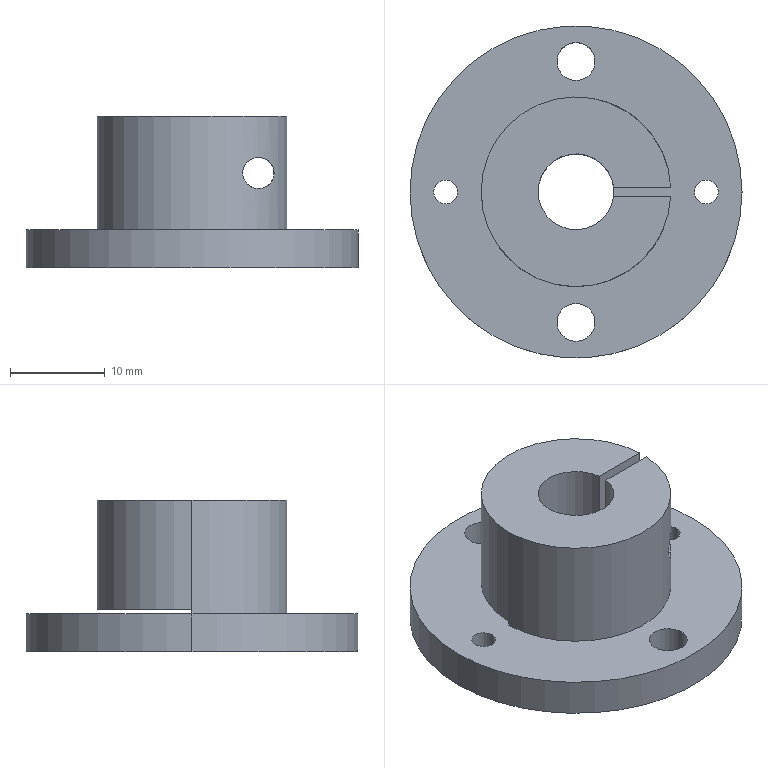Part | STEP file | 11-FG-B04611 | 1 solid | 30 faces | box 35 x 35 x 16 mm | volume 6298 mm3 | cylinder 22 | plane 8 | commonest cylinder face diameters 8 x6 2.5 x4 4 x4 3.3 x2 4.5 x2 20 x2
STEP:
#1=CARTESIAN_POINT('',(12.5,0.,4.));
#2=VERTEX_POINT('',#1);
#3=CARTESIAN_POINT('',(15.,0.,4.));
#4=VERTEX_POINT('',#3);
#5=CARTESIAN_POINT('',(13.75,0.,4.));
#6=DIRECTION('',(0.,0.,1.));
#7=DIRECTION('',(1.,0.,0.));
#8=AXIS2_PLACEMENT_3D('',#5,#6,#7);
#9=CIRCLE('',#8,1.25);
#10=EDGE_CURVE('',#2,#4,#9,.T.);
#11=ORIENTED_EDGE('',*,*,#10,.T.);
#12=CARTESIAN_POINT('',(15.,0.,0.));
#13=VERTEX_POINT('',#12);
#14=CARTESIAN_POINT('',(15.,0.,0.));
#15=DIRECTION('',(0.,0.,-1.));
#16=VECTOR('',#15,1000.);
#17=LINE('',#14,#16);
#18=EDGE_CURVE('',#4,#13,#17,.T.);
#19=ORIENTED_EDGE('',*,*,#18,.T.);
#20=CARTESIAN_POINT('',(12.5,0.,0.));
#21=VERTEX_POINT('',#20);
#22=CARTESIAN_POINT('',(13.75,0.,0.));
#23=DIRECTION('',(0.,0.,-1.));
#24=DIRECTION('',(-1.,0.,0.));
#25=AXIS2_PLACEMENT_3D('',#22,#23,#24);
#26=CIRCLE('',#25,1.25);
#27=EDGE_CURVE('',#13,#21,#26,.T.);
#28=ORIENTED_EDGE('',*,*,#27,.T.);
#29=CARTESIAN_POINT('',(12.5,0.,0.));
#30=DIRECTION('',(0.,0.,-1.));
#31=VECTOR('',#30,1000.);
#32=LINE('',#29,#31);
#33=EDGE_CURVE('',#2,#21,#32,.T.);
#34=ORIENTED_EDGE('',*,*,#33,.F.);
#35=EDGE_LOOP('',(#11,#19,#28,#34));
#36=FACE_OUTER_BOUND('',#35,.T.);
#37=CARTESIAN_POINT('',(13.75,0.,0.));
#38=DIRECTION('',(0.,0.,-1.));
#39=DIRECTION('',(-1.,0.,0.));
#40=AXIS2_PLACEMENT_3D('',#37,#38,#39);
#41=CYLINDRICAL_SURFACE('',#40,1.25);
#42=ADVANCED_FACE('',(#36),#41,.F.);
#43=CARTESIAN_POINT('',(-15.,0.,4.));
#44=VERTEX_POINT('',#43);
#45=CARTESIAN_POINT('',(-12.5,0.,4.));
#46=VERTEX_POINT('',#45);
#47=CARTESIAN_POINT('',(-13.75,0.,4.));
#48=DIRECTION('',(0.,0.,1.));
#49=DIRECTION('',(1.,0.,0.));
#50=AXIS2_PLACEMENT_3D('',#47,#48,#49);
#51=CIRCLE('',#50,1.25);
#52=EDGE_CURVE('',#44,#46,#51,.T.);
#53=ORIENTED_EDGE('',*,*,#52,.T.);
#54=CARTESIAN_POINT('',(-12.5,0.,0.));
#55=VERTEX_POINT('',#54);
#56=CARTESIAN_POINT('',(-12.5,0.,0.));
#57=DIRECTION('',(0.,0.,-1.));
#58=VECTOR('',#57,1000.);
#59=LINE('',#56,#58);
#60=EDGE_CURVE('',#46,#55,#59,.T.);
#61=ORIENTED_EDGE('',*,*,#60,.T.);
#62=CARTESIAN_POINT('',(-15.,0.,0.));
#63=VERTEX_POINT('',#62);
#64=CARTESIAN_POINT('',(-13.75,0.,0.));
#65=DIRECTION('',(0.,0.,-1.));
#66=DIRECTION('',(-1.,0.,0.));
#67=AXIS2_PLACEMENT_3D('',#64,#65,#66);
#68=CIRCLE('',#67,1.25);
#69=EDGE_CURVE('',#55,#63,#68,.T.);
#70=ORIENTED_EDGE('',*,*,#69,.T.);
#71=CARTESIAN_POINT('',(-15.,0.,0.));
#72=DIRECTION('',(0.,0.,-1.));
#73=VECTOR('',#72,1000.);
#74=LINE('',#71,#73);
#75=EDGE_CURVE('',#44,#63,#74,.T.);
#76=ORIENTED_EDGE('',*,*,#75,.F.);
#77=EDGE_LOOP('',(#53,#61,#70,#76));
#78=FACE_OUTER_BOUND('',#77,.T.);
#79=CARTESIAN_POINT('',(-13.75,0.,0.));
#80=DIRECTION('',(0.,0.,-1.));
#81=DIRECTION('',(-1.,0.,0.));
#82=AXIS2_PLACEMENT_3D('',#79,#80,#81);
#83=CYLINDRICAL_SURFACE('',#82,1.25);
#84=ADVANCED_FACE('',(#78),#83,.F.);
#85=CARTESIAN_POINT('',(-2.,-13.75,0.));
#86=VERTEX_POINT('',#85);
#87=CARTESIAN_POINT('',(2.,-13.75,0.));
#88=VERTEX_POINT('',#87);
#89=CARTESIAN_POINT('',(0.,-13.75,0.));
#90=DIRECTION('',(0.,0.,1.));
#91=DIRECTION('',(1.,0.,0.));
#92=AXIS2_PLACEMENT_3D('',#89,#90,#91);
#93=CIRCLE('',#92,2.);
#94=EDGE_CURVE('',#86,#88,#93,.T.);
#95=ORIENTED_EDGE('',*,*,#94,.F.);
#96=CARTESIAN_POINT('',(-2.,-13.75,4.));
#97=VERTEX_POINT('',#96);
#98=CARTESIAN_POINT('',(-2.,-13.75,-15.));
#99=DIRECTION('',(0.,0.,1.));
#100=VECTOR('',#99,1000.);
#101=LINE('',#98,#100);
#102=EDGE_CURVE('',#86,#97,#101,.T.);
#103=ORIENTED_EDGE('',*,*,#102,.T.);
#104=CARTESIAN_POINT('',(2.,-13.75,4.));
#105=VERTEX_POINT('',#104);
#106=CARTESIAN_POINT('',(0.,-13.75,4.));
#107=DIRECTION('',(0.,0.,1.));
#108=DIRECTION('',(1.,0.,0.));
#109=AXIS2_PLACEMENT_3D('',#106,#107,#108);
#110=CIRCLE('',#109,2.);
#111=EDGE_CURVE('',#97,#105,#110,.T.);
#112=ORIENTED_EDGE('',*,*,#111,.T.);
#113=CARTESIAN_POINT('',(2.,-13.75,-15.));
#114=DIRECTION('',(0.,0.,1.));
#115=VECTOR('',#114,1000.);
#116=LINE('',#113,#115);
#117=EDGE_CURVE('',#88,#105,#116,.T.);
#118=ORIENTED_EDGE('',*,*,#117,.F.);
#119=EDGE_LOOP('',(#95,#103,#112,#118));
#120=FACE_OUTER_BOUND('',#119,.T.);
#121=CARTESIAN_POINT('',(0.,-13.75,-15.));
#122=DIRECTION('',(0.,0.,1.));
#123=DIRECTION('',(1.,0.,0.));
#124=AXIS2_PLACEMENT_3D('',#121,#122,#123);
#125=CYLINDRICAL_SURFACE('',#124,2.);
#126=ADVANCED_FACE('',(#120),#125,.F.);
#127=CARTESIAN_POINT('',(-2.,13.75,0.));
#128=VERTEX_POINT('',#127);
#129=CARTESIAN_POINT('',(2.,13.75,0.));
#130=VERTEX_POINT('',#129);
#131=CARTESIAN_POINT('',(0.,13.75,0.));
#132=DIRECTION('',(0.,0.,1.));
#133=DIRECTION('',(1.,0.,0.));
#134=AXIS2_PLACEMENT_3D('',#131,#132,#133);
#135=CIRCLE('',#134,2.);
#136=EDGE_CURVE('',#128,#130,#135,.T.);
#137=ORIENTED_EDGE('',*,*,#136,.F.);
#138=CARTESIAN_POINT('',(-2.,13.75,4.));
#139=VERTEX_POINT('',#138);
#140=CARTESIAN_POINT('',(-2.,13.75,-15.));
#141=DIRECTION('',(0.,0.,1.));
#142=VECTOR('',#141,1000.);
#143=LINE('',#140,#142);
#144=EDGE_CURVE('',#128,#139,#143,.T.);
#145=ORIENTED_EDGE('',*,*,#144,.T.);
#146=CARTESIAN_POINT('',(2.,13.75,4.));
#147=VERTEX_POINT('',#146);
#148=CARTESIAN_POINT('',(0.,13.75,4.));
#149=DIRECTION('',(0.,0.,1.));
#150=DIRECTION('',(1.,0.,0.));
#151=AXIS2_PLACEMENT_3D('',#148,#149,#150);
#152=CIRCLE('',#151,2.);
#153=EDGE_CURVE('',#139,#147,#152,.T.);
#154=ORIENTED_EDGE('',*,*,#153,.T.);
#155=CARTESIAN_POINT('',(2.,13.75,-15.));
#156=DIRECTION('',(0.,0.,1.));
#157=VECTOR('',#156,1000.);
#158=LINE('',#155,#157);
#159=EDGE_CURVE('',#130,#147,#158,.T.);
#160=ORIENTED_EDGE('',*,*,#159,.F.);
#161=EDGE_LOOP('',(#137,#145,#154,#160));
#162=FACE_OUTER_BOUND('',#161,.T.);
#163=CARTESIAN_POINT('',(0.,13.75,-15.));
#164=DIRECTION('',(0.,0.,1.));
#165=DIRECTION('',(1.,0.,0.));
#166=AXIS2_PLACEMENT_3D('',#163,#164,#165);
#167=CYLINDRICAL_SURFACE('',#166,2.);
#168=ADVANCED_FACE('',(#162),#167,.F.);
#169=CARTESIAN_POINT('',(17.5,0.,4.));
#170=VERTEX_POINT('',#169);
#171=CARTESIAN_POINT('',(-17.5,0.,4.));
#172=VERTEX_POINT('',#171);
#173=CARTESIAN_POINT('',(0.,0.,4.));
#174=DIRECTION('',(0.,0.,1.));
#175=DIRECTION('',(1.,0.,0.));
#176=AXIS2_PLACEMENT_3D('',#173,#174,#175);
#177=CIRCLE('',#176,17.5);
#178=EDGE_CURVE('',#170,#172,#177,.T.);
#179=ORIENTED_EDGE('',*,*,#178,.F.);
#180=CARTESIAN_POINT('',(17.5,0.,0.));
#181=VERTEX_POINT('',#180);
#182=CARTESIAN_POINT('',(17.5,0.,24.));
#183=DIRECTION('',(0.,0.,-1.));
#184=VECTOR('',#183,1000.);
#185=LINE('',#182,#184);
#186=EDGE_CURVE('',#170,#181,#185,.T.);
#187=ORIENTED_EDGE('',*,*,#186,.T.);
#188=CARTESIAN_POINT('',(-17.5,0.,0.));
#189=VERTEX_POINT('',#188);
#190=CARTESIAN_POINT('',(0.,0.,0.));
#191=DIRECTION('',(0.,0.,-1.));
#192=DIRECTION('',(-1.,0.,0.));
#193=AXIS2_PLACEMENT_3D('',#190,#191,#192);
#194=CIRCLE('',#193,17.5);
#195=EDGE_CURVE('',#189,#181,#194,.T.);
#196=ORIENTED_EDGE('',*,*,#195,.F.);
#197=CARTESIAN_POINT('',(-17.5,0.,24.));
#198=DIRECTION('',(0.,0.,-1.));
#199=VECTOR('',#198,1000.);
#200=LINE('',#197,#199);
#201=EDGE_CURVE('',#172,#189,#200,.T.);
#202=ORIENTED_EDGE('',*,*,#201,.F.);
#203=EDGE_LOOP('',(#179,#187,#196,#202));
#204=FACE_OUTER_BOUND('',#203,.T.);
#205=CARTESIAN_POINT('',(0.,0.,24.));
#206=DIRECTION('',(0.,0.,-1.));
#207=DIRECTION('',(-1.,0.,0.));
#208=AXIS2_PLACEMENT_3D('',#205,#206,#207);
#209=CYLINDRICAL_SURFACE('',#208,17.5);
#210=ADVANCED_FACE('',(#204),#209,.T.);
#211=CARTESIAN_POINT('',(7.,-7.141,8.35));
#212=VERTEX_POINT('',#211);
#213=CARTESIAN_POINT('',(7.,-7.141,11.65));
#214=VERTEX_POINT('',#213);
#215=CARTESIAN_POINT('',(7.,-7.141,8.35));
#216=CARTESIAN_POINT('',(6.823,-7.315,8.35));
#217=CARTESIAN_POINT('',(6.639,-7.482,8.378));
#218=CARTESIAN_POINT('',(6.366,-7.713,8.474));
#219=CARTESIAN_POINT('',(6.273,-7.788,8.515));
#220=CARTESIAN_POINT('',(6.096,-7.928,8.616));
#221=CARTESIAN_POINT('',(6.01,-7.993,8.676));
#222=CARTESIAN_POINT('',(5.762,-8.175,8.887));
#223=CARTESIAN_POINT('',(5.616,-8.275,9.071));
#224=CARTESIAN_POINT('',(5.461,-8.378,9.394));
#225=CARTESIAN_POINT('',(5.42,-8.404,9.508));
#226=CARTESIAN_POINT('',(5.365,-8.439,9.747));
#227=CARTESIAN_POINT('',(5.35,-8.448,9.872));
#228=CARTESIAN_POINT('',(5.35,-8.449,10.12));
#229=CARTESIAN_POINT('',(5.364,-8.44,10.246));
#230=CARTESIAN_POINT('',(5.418,-8.405,10.485));
#231=CARTESIAN_POINT('',(5.459,-8.379,10.601));
#232=CARTESIAN_POINT('',(5.614,-8.277,10.926));
#233=CARTESIAN_POINT('',(5.76,-8.177,11.11));
#234=CARTESIAN_POINT('',(6.006,-7.996,11.322));
#235=CARTESIAN_POINT('',(6.094,-7.929,11.383));
#236=CARTESIAN_POINT('',(6.272,-7.789,11.484));
#237=CARTESIAN_POINT('',(6.362,-7.716,11.525));
#238=CARTESIAN_POINT('',(6.636,-7.485,11.621));
#239=CARTESIAN_POINT('',(6.822,-7.316,11.65));
#240=CARTESIAN_POINT('',(7.,-7.141,11.65));
#241=B_SPLINE_CURVE_WITH_KNOTS('',3,(#215,#216,#217,#218,#219,#220,#221,#222,#223,#224,#225,#226,#227,#228,#229,#230,#231,#232,#233,#234,#235,#236,#237,#238,#239,#240),.UNSPECIFIED.,.F.,.F.,(4,2,2,2,2,2,2,2,2,2,2,2,4),(0.006793,0.00753,0.007898,0.008266,0.009003,0.009371,0.009739,0.01011,0.01048,0.01121,0.01158,0.01195,0.01269),.UNSPECIFIED.);
#242=EDGE_CURVE('',#212,#214,#241,.T.);
#243=ORIENTED_EDGE('',*,*,#242,.F.);
#244=CARTESIAN_POINT('',(7.,-0.5,8.35));
#245=VERTEX_POINT('',#244);
#246=CARTESIAN_POINT('',(7.,-0.5,8.35));
#247=DIRECTION('',(0.,1.,0.));
#248=VECTOR('',#247,1000.);
#249=LINE('',#246,#248);
#250=EDGE_CURVE('',#212,#245,#249,.T.);
#251=ORIENTED_EDGE('',*,*,#250,.T.);
#252=CARTESIAN_POINT('',(7.,-0.5,11.65));
#253=VERTEX_POINT('',#252);
#254=CARTESIAN_POINT('',(7.,-0.5,10.));
#255=DIRECTION('',(0.,1.,0.));
#256=DIRECTION('',(0.,0.,1.));
#257=AXIS2_PLACEMENT_3D('',#254,#255,#256);
#258=CIRCLE('',#257,1.65);
#259=EDGE_CURVE('',#245,#253,#258,.T.);
#260=ORIENTED_EDGE('',*,*,#259,.T.);
#261=CARTESIAN_POINT('',(7.,-0.5,11.65));
#262=DIRECTION('',(0.,1.,0.));
#263=VECTOR('',#262,1000.);
#264=LINE('',#261,#263);
#265=EDGE_CURVE('',#214,#253,#264,.T.);
#266=ORIENTED_EDGE('',*,*,#265,.F.);
#267=EDGE_LOOP('',(#243,#251,#260,#266));
#268=FACE_OUTER_BOUND('',#267,.T.);
#269=CARTESIAN_POINT('',(7.,-0.5,10.));
#270=DIRECTION('',(0.,1.,0.));
#271=DIRECTION('',(0.,0.,1.));
#272=AXIS2_PLACEMENT_3D('',#269,#270,#271);
#273=CYLINDRICAL_SURFACE('',#272,1.65);
#274=ADVANCED_FACE('',(#268),#273,.F.);
#275=CARTESIAN_POINT('',(7.,4.5,6.));
#276=VERTEX_POINT('',#275);
#277=CARTESIAN_POINT('',(7.,4.5,14.));
#278=VERTEX_POINT('',#277);
#279=CARTESIAN_POINT('',(7.,4.5,10.));
#280=DIRECTION('',(0.,1.,0.));
#281=DIRECTION('',(0.,0.,1.));
#282=AXIS2_PLACEMENT_3D('',#279,#280,#281);
#283=CIRCLE('',#282,4.);
#284=EDGE_CURVE('',#276,#278,#283,.T.);
#285=ORIENTED_EDGE('',*,*,#284,.F.);
#286=CARTESIAN_POINT('',(7.,7.141,6.));
#287=VERTEX_POINT('',#286);
#288=CARTESIAN_POINT('',(7.,4.5,6.));
#289=DIRECTION('',(0.,1.,0.));
#290=VECTOR('',#289,1000.);
#291=LINE('',#288,#290);
#292=EDGE_CURVE('',#276,#287,#291,.T.);
#293=ORIENTED_EDGE('',*,*,#292,.T.);
#294=CARTESIAN_POINT('',(7.,7.141,14.));
#295=VERTEX_POINT('',#294);
#296=CARTESIAN_POINT('',(7.,7.141,14.));
#297=CARTESIAN_POINT('',(6.794,7.343,14.));
#298=CARTESIAN_POINT('',(6.581,7.535,13.984));
#299=CARTESIAN_POINT('',(6.141,7.897,13.913));
#300=CARTESIAN_POINT('',(5.912,8.07,13.857));
#301=CARTESIAN_POINT('',(5.457,8.384,13.698));
#302=CARTESIAN_POINT('',(5.231,8.526,13.597));
#303=CARTESIAN_POINT('',(4.899,8.719,13.406));
#304=CARTESIAN_POINT('',(4.79,8.779,13.336));
#305=CARTESIAN_POINT('',(4.573,8.894,13.182));
#306=CARTESIAN_POINT('',(4.466,8.948,13.098));
#307=CARTESIAN_POINT('',(4.161,9.096,12.831));
#308=CARTESIAN_POINT('',(3.974,9.178,12.631));
#309=CARTESIAN_POINT('',(3.638,9.317,12.184));
#310=CARTESIAN_POINT('',(3.489,9.373,11.937));
#311=CARTESIAN_POINT('',(3.25,9.458,11.421));
#312=CARTESIAN_POINT('',(3.157,9.489,11.148));
#313=CARTESIAN_POINT('',(3.032,9.529,10.583));
#314=CARTESIAN_POINT('',(3.001,9.539,10.297));
#315=CARTESIAN_POINT('',(2.999,9.54,9.72));
#316=CARTESIAN_POINT('',(3.031,9.53,9.428));
#317=CARTESIAN_POINT('',(3.153,9.49,8.868));
#318=CARTESIAN_POINT('',(3.245,9.46,8.593));
#319=CARTESIAN_POINT('',(3.483,9.375,8.072));
#320=CARTESIAN_POINT('',(3.628,9.32,7.83));
#321=CARTESIAN_POINT('',(3.964,9.183,7.381));
#322=CARTESIAN_POINT('',(4.155,9.099,7.175));
#323=CARTESIAN_POINT('',(4.561,8.902,6.818));
#324=CARTESIAN_POINT('',(4.779,8.788,6.663));
#325=CARTESIAN_POINT('',(5.228,8.528,6.404));
#326=CARTESIAN_POINT('',(5.456,8.385,6.302));
#327=CARTESIAN_POINT('',(5.913,8.069,6.143));
#328=CARTESIAN_POINT('',(6.142,7.897,6.087));
#329=CARTESIAN_POINT('',(6.581,7.534,6.016));
#330=CARTESIAN_POINT('',(6.794,7.343,6.));
#331=CARTESIAN_POINT('',(7.,7.141,6.));
#332=B_SPLINE_CURVE_WITH_KNOTS('',3,(#296,#297,#298,#299,#300,#301,#302,#303,#304,#305,#306,#307,#308,#309,#310,#311,#312,#313,#314,#315,#316,#317,#318,#319,#320,#321,#322,#323,#324,#325,#326,#327,#328,#329,#330,#331),.UNSPECIFIED.,.F.,.F.,(4,2,2,2,2,2,2,2,2,2,2,2,2,2,2,2,2,4),(0.00331,0.004163,0.005015,0.005867,0.006294,0.00672,0.007572,0.008425,0.009277,0.01013,0.01098,0.01183,0.01269,0.01354,0.01439,0.01524,0.0161,0.01695),.UNSPECIFIED.);
#333=EDGE_CURVE('',#295,#287,#332,.T.);
#334=ORIENTED_EDGE('',*,*,#333,.F.);
#335=CARTESIAN_POINT('',(7.,4.5,14.));
#336=DIRECTION('',(0.,1.,0.));
#337=VECTOR('',#336,1000.);
#338=LINE('',#335,#337);
#339=EDGE_CURVE('',#278,#295,#338,.T.);
#340=ORIENTED_EDGE('',*,*,#339,.F.);
#341=EDGE_LOOP('',(#285,#293,#334,#340));
#342=FACE_OUTER_BOUND('',#341,.T.);
#343=CARTESIAN_POINT('',(7.,4.5,10.));
#344=DIRECTION('',(0.,1.,0.));
#345=DIRECTION('',(0.,0.,1.));
#346=AXIS2_PLACEMENT_3D('',#343,#344,#345);
#347=CYLINDRICAL_SURFACE('',#346,4.);
#348=ADVANCED_FACE('',(#342),#347,.F.);
#349=CARTESIAN_POINT('',(8.93,4.5,13.503));
#350=VERTEX_POINT('',#349);
#351=CARTESIAN_POINT('',(7.,4.5,10.));
#352=DIRECTION('',(0.,1.,0.));
#353=DIRECTION('',(0.,0.,1.));
#354=AXIS2_PLACEMENT_3D('',#351,#352,#353);
#355=CIRCLE('',#354,4.);
#356=EDGE_CURVE('',#278,#350,#355,.T.);
#357=ORIENTED_EDGE('',*,*,#356,.F.);
#358=ORIENTED_EDGE('',*,*,#339,.T.);
#359=CARTESIAN_POINT('',(8.93,4.5,13.503));
#360=CARTESIAN_POINT('',(8.686,4.985,13.638));
#361=CARTESIAN_POINT('',(8.404,5.446,13.76));
#362=CARTESIAN_POINT('',(7.924,6.107,13.895));
#363=CARTESIAN_POINT('',(7.754,6.321,13.933));
#364=CARTESIAN_POINT('',(7.393,6.74,13.985));
#365=CARTESIAN_POINT('',(7.2,6.945,14.));
#366=CARTESIAN_POINT('',(7.,7.141,14.));
#367=B_SPLINE_CURVE_WITH_KNOTS('',3,(#359,#360,#361,#362,#363,#364,#365,#366),.UNSPECIFIED.,.F.,.F.,(4,2,2,4),(0.,0.001655,0.002483,0.00331),.UNSPECIFIED.);
#368=EDGE_CURVE('',#350,#295,#367,.T.);
#369=ORIENTED_EDGE('',*,*,#368,.F.);
#370=EDGE_LOOP('',(#357,#358,#369));
#371=FACE_OUTER_BOUND('',#370,.T.);
#372=CARTESIAN_POINT('',(7.,4.5,10.));
#373=DIRECTION('',(0.,1.,0.));
#374=DIRECTION('',(0.,0.,1.));
#375=AXIS2_PLACEMENT_3D('',#372,#373,#374);
#376=CYLINDRICAL_SURFACE('',#375,4.);
#377=ADVANCED_FACE('',(#371),#376,.F.);
#378=CARTESIAN_POINT('',(-4.,0.,0.));
#379=VERTEX_POINT('',#378);
#380=CARTESIAN_POINT('',(4.,0.,0.));
#381=VERTEX_POINT('',#380);
#382=CARTESIAN_POINT('',(0.,0.,0.));
#383=DIRECTION('',(0.,0.,1.));
#384=DIRECTION('',(1.,0.,0.));
#385=AXIS2_PLACEMENT_3D('',#382,#383,#384);
#386=CIRCLE('',#385,4.);
#387=EDGE_CURVE('',#379,#381,#386,.T.);
#388=ORIENTED_EDGE('',*,*,#387,.F.);
#389=CARTESIAN_POINT('',(-4.,0.,4.));
#390=VERTEX_POINT('',#389);
#391=CARTESIAN_POINT('',(-4.,0.,0.));
#392=DIRECTION('',(0.,0.,1.));
#393=VECTOR('',#392,1000.);
#394=LINE('',#391,#393);
#395=EDGE_CURVE('',#379,#390,#394,.T.);
#396=ORIENTED_EDGE('',*,*,#395,.T.);
#397=CARTESIAN_POINT('',(-4.,0.,4.5));
#398=VERTEX_POINT('',#397);
#399=CARTESIAN_POINT('',(-4.,0.,0.));
#400=DIRECTION('',(0.,0.,1.));
#401=VECTOR('',#400,1000.);
#402=LINE('',#399,#401);
#403=EDGE_CURVE('',#390,#398,#402,.T.);
#404=ORIENTED_EDGE('',*,*,#403,.T.);
#405=CARTESIAN_POINT('',(-4.,0.,16.));
#406=VERTEX_POINT('',#405);
#407=CARTESIAN_POINT('',(-4.,0.,0.));
#408=DIRECTION('',(0.,0.,1.));
#409=VECTOR('',#408,1000.);
#410=LINE('',#407,#409);
#411=EDGE_CURVE('',#398,#406,#410,.T.);
#412=ORIENTED_EDGE('',*,*,#411,.T.);
#413=CARTESIAN_POINT('',(3.969,-0.5,16.));
#414=VERTEX_POINT('',#413);
#415=CARTESIAN_POINT('',(0.,0.,16.));
#416=DIRECTION('',(0.,0.,1.));
#417=DIRECTION('',(1.,0.,0.));
#418=AXIS2_PLACEMENT_3D('',#415,#416,#417);
#419=CIRCLE('',#418,4.);
#420=EDGE_CURVE('',#406,#414,#419,.T.);
#421=ORIENTED_EDGE('',*,*,#420,.T.);
#422=CARTESIAN_POINT('',(3.969,-0.5,4.));
#423=VERTEX_POINT('',#422);
#424=CARTESIAN_POINT('',(3.969,-0.5,0.));
#425=DIRECTION('',(0.,0.,-1.));
#426=VECTOR('',#425,1000.);
#427=LINE('',#424,#426);
#428=EDGE_CURVE('',#414,#423,#427,.T.);
#429=ORIENTED_EDGE('',*,*,#428,.T.);
#430=CARTESIAN_POINT('',(4.,0.,4.));
#431=VERTEX_POINT('',#430);
#432=CARTESIAN_POINT('',(0.,0.,4.));
#433=DIRECTION('',(0.,0.,-1.));
#434=DIRECTION('',(1.,0.,0.));
#435=AXIS2_PLACEMENT_3D('',#432,#433,#434);
#436=CIRCLE('',#435,4.);
#437=EDGE_CURVE('',#431,#423,#436,.T.);
#438=ORIENTED_EDGE('',*,*,#437,.F.);
#439=CARTESIAN_POINT('',(4.,0.,0.));
#440=DIRECTION('',(0.,0.,1.));
#441=VECTOR('',#440,1000.);
#442=LINE('',#439,#441);
#443=EDGE_CURVE('',#381,#431,#442,.T.);
#444=ORIENTED_EDGE('',*,*,#443,.F.);
#445=EDGE_LOOP('',(#388,#396,#404,#412,#421,#429,#438,#444));
#446=FACE_OUTER_BOUND('',#445,.T.);
#447=CARTESIAN_POINT('',(0.,0.,0.));
#448=DIRECTION('',(0.,0.,1.));
#449=DIRECTION('',(1.,0.,0.));
#450=AXIS2_PLACEMENT_3D('',#447,#448,#449);
#451=CYLINDRICAL_SURFACE('',#450,4.);
#452=ADVANCED_FACE('',(#446),#451,.F.);
#453=ORIENTED_EDGE('',*,*,#395,.F.);
#454=CARTESIAN_POINT('',(0.,0.,0.));
#455=DIRECTION('',(0.,0.,1.));
#456=DIRECTION('',(1.,0.,0.));
#457=AXIS2_PLACEMENT_3D('',#454,#455,#456);
#458=CIRCLE('',#457,4.);
#459=EDGE_CURVE('',#381,#379,#458,.T.);
#460=ORIENTED_EDGE('',*,*,#459,.F.);
#461=ORIENTED_EDGE('',*,*,#443,.T.);
#462=CARTESIAN_POINT('',(0.,0.,4.));
#463=DIRECTION('',(0.,0.,-1.));
#464=DIRECTION('',(1.,0.,0.));
#465=AXIS2_PLACEMENT_3D('',#462,#463,#464);
#466=CIRCLE('',#465,4.);
#467=EDGE_CURVE('',#390,#431,#466,.T.);
#468=ORIENTED_EDGE('',*,*,#467,.F.);
#469=EDGE_LOOP('',(#453,#460,#461,#468));
#470=FACE_OUTER_BOUND('',#469,.T.);
#471=CARTESIAN_POINT('',(0.,0.,0.));
#472=DIRECTION('',(0.,0.,1.));
#473=DIRECTION('',(1.,0.,0.));
#474=AXIS2_PLACEMENT_3D('',#471,#472,#473);
#475=CYLINDRICAL_SURFACE('',#474,4.);
#476=ADVANCED_FACE('',(#470),#475,.F.);
#477=CARTESIAN_POINT('',(7.,4.5,12.25));
#478=VERTEX_POINT('',#477);
#479=CARTESIAN_POINT('',(7.,4.5,7.75));
#480=VERTEX_POINT('',#479);
#481=CARTESIAN_POINT('',(7.,4.5,10.));
#482=DIRECTION('',(0.,-1.,0.));
#483=DIRECTION('',(0.,0.,1.));
#484=AXIS2_PLACEMENT_3D('',#481,#482,#483);
#485=CIRCLE('',#484,2.25);
#486=EDGE_CURVE('',#478,#480,#485,.T.);
#487=ORIENTED_EDGE('',*,*,#486,.F.);
#488=CARTESIAN_POINT('',(7.,0.5,12.25));
#489=VERTEX_POINT('',#488);
#490=CARTESIAN_POINT('',(7.,31.441,12.25));
#491=DIRECTION('',(0.,-1.,0.));
#492=VECTOR('',#491,1000.);
#493=LINE('',#490,#492);
#494=EDGE_CURVE('',#478,#489,#493,.T.);
#495=ORIENTED_EDGE('',*,*,#494,.T.);
#496=CARTESIAN_POINT('',(7.,0.5,7.75));
#497=VERTEX_POINT('',#496);
#498=CARTESIAN_POINT('',(7.,0.5,10.));
#499=DIRECTION('',(0.,-1.,0.));
#500=DIRECTION('',(0.,0.,-1.));
#501=AXIS2_PLACEMENT_3D('',#498,#499,#500);
#502=CIRCLE('',#501,2.25);
#503=EDGE_CURVE('',#489,#497,#502,.T.);
#504=ORIENTED_EDGE('',*,*,#503,.T.);
#505=CARTESIAN_POINT('',(7.,31.441,7.75));
#506=DIRECTION('',(0.,-1.,0.));
#507=VECTOR('',#506,1000.);
#508=LINE('',#505,#507);
#509=EDGE_CURVE('',#480,#497,#508,.T.);
#510=ORIENTED_EDGE('',*,*,#509,.F.);
#511=EDGE_LOOP('',(#487,#495,#504,#510));
#512=FACE_OUTER_BOUND('',#511,.T.);
#513=CARTESIAN_POINT('',(7.,31.441,10.));
#514=DIRECTION('',(0.,-1.,0.));
#515=DIRECTION('',(0.,0.,-1.));
#516=AXIS2_PLACEMENT_3D('',#513,#514,#515);
#517=CYLINDRICAL_SURFACE('',#516,2.25);
#518=ADVANCED_FACE('',(#512),#517,.F.);
#519=CARTESIAN_POINT('',(7.,-7.141,11.65));
#520=CARTESIAN_POINT('',(7.205,-6.94,11.65));
#521=CARTESIAN_POINT('',(7.397,-6.735,11.613));
#522=CARTESIAN_POINT('',(7.757,-6.317,11.479));
#523=CARTESIAN_POINT('',(7.925,-6.104,11.38));
#524=CARTESIAN_POINT('',(8.148,-5.798,11.189));
#525=CARTESIAN_POINT('',(8.218,-5.698,11.118));
#526=CARTESIAN_POINT('',(8.35,-5.504,10.955));
#527=CARTESIAN_POINT('',(8.411,-5.41,10.863));
#528=CARTESIAN_POINT('',(8.517,-5.241,10.658));
#529=CARTESIAN_POINT('',(8.564,-5.164,10.543));
#530=CARTESIAN_POINT('',(8.63,-5.053,10.29));
#531=CARTESIAN_POINT('',(8.65,-5.018,10.147));
#532=CARTESIAN_POINT('',(8.65,-5.017,9.858));
#533=CARTESIAN_POINT('',(8.631,-5.051,9.715));
#534=CARTESIAN_POINT('',(8.565,-5.163,9.46));
#535=CARTESIAN_POINT('',(8.518,-5.239,9.344));
#536=CARTESIAN_POINT('',(8.359,-5.492,9.037));
#537=CARTESIAN_POINT('',(8.224,-5.694,8.876));
#538=CARTESIAN_POINT('',(7.925,-6.104,8.62));
#539=CARTESIAN_POINT('',(7.758,-6.316,8.522));
#540=CARTESIAN_POINT('',(7.396,-6.736,8.387));
#541=CARTESIAN_POINT('',(7.204,-6.941,8.35));
#542=CARTESIAN_POINT('',(7.,-7.141,8.35));
#543=B_SPLINE_CURVE_WITH_KNOTS('',3,(#519,#520,#521,#522,#523,#524,#525,#526,#527,#528,#529,#530,#531,#532,#533,#534,#535,#536,#537,#538,#539,#540,#541,#542),.UNSPECIFIED.,.F.,.F.,(4,2,2,2,2,2,2,2,2,2,2,4),(0.,0.0008492,0.001698,0.002123,0.002547,0.002972,0.003397,0.003821,0.004246,0.005095,0.005944,0.006793),.UNSPECIFIED.);
#544=EDGE_CURVE('',#214,#212,#543,.T.);
#545=ORIENTED_EDGE('',*,*,#544,.T.);
#546=ORIENTED_EDGE('',*,*,#242,.T.);
#547=EDGE_LOOP('',(#545,#546));
#548=FACE_BOUND('',#547,.T.);
#549=CARTESIAN_POINT('',(-10.,0.,16.));
#550=VERTEX_POINT('',#549);
#551=CARTESIAN_POINT('',(9.987,-0.5,16.));
#552=VERTEX_POINT('',#551);
#553=CARTESIAN_POINT('',(0.,0.,16.));
#554=DIRECTION('',(0.,0.,1.));
#555=DIRECTION('',(1.,0.,0.));
#556=AXIS2_PLACEMENT_3D('',#553,#554,#555);
#557=CIRCLE('',#556,10.);
#558=EDGE_CURVE('',#550,#552,#557,.T.);
#559=ORIENTED_EDGE('',*,*,#558,.F.);
#560=CARTESIAN_POINT('',(-10.,0.,4.5));
#561=VERTEX_POINT('',#560);
#562=CARTESIAN_POINT('',(-10.,0.,16.));
#563=DIRECTION('',(0.,0.,-1.));
#564=VECTOR('',#563,1000.);
#565=LINE('',#562,#564);
#566=EDGE_CURVE('',#550,#561,#565,.T.);
#567=ORIENTED_EDGE('',*,*,#566,.T.);
#568=CARTESIAN_POINT('',(-10.,0.,4.));
#569=VERTEX_POINT('',#568);
#570=CARTESIAN_POINT('',(-10.,0.,16.));
#571=DIRECTION('',(0.,0.,-1.));
#572=VECTOR('',#571,1000.);
#573=LINE('',#570,#572);
#574=EDGE_CURVE('',#561,#569,#573,.T.);
#575=ORIENTED_EDGE('',*,*,#574,.T.);
#576=CARTESIAN_POINT('',(9.987,-0.5,4.));
#577=VERTEX_POINT('',#576);
#578=CARTESIAN_POINT('',(0.,0.,4.));
#579=DIRECTION('',(0.,0.,1.));
#580=DIRECTION('',(1.,0.,0.));
#581=AXIS2_PLACEMENT_3D('',#578,#579,#580);
#582=CIRCLE('',#581,10.);
#583=EDGE_CURVE('',#569,#577,#582,.T.);
#584=ORIENTED_EDGE('',*,*,#583,.T.);
#585=CARTESIAN_POINT('',(9.987,-0.5,16.));
#586=DIRECTION('',(0.,0.,1.));
#587=VECTOR('',#586,1000.);
#588=LINE('',#585,#587);
#589=EDGE_CURVE('',#577,#552,#588,.T.);
#590=ORIENTED_EDGE('',*,*,#589,.T.);
#591=EDGE_LOOP('',(#559,#567,#575,#584,#590));
#592=FACE_OUTER_BOUND('',#591,.T.);
#593=CARTESIAN_POINT('',(0.,0.,16.));
#594=DIRECTION('',(0.,0.,-1.));
#595=DIRECTION('',(-1.,0.,0.));
#596=AXIS2_PLACEMENT_3D('',#593,#594,#595);
#597=CYLINDRICAL_SURFACE('',#596,10.);
#598=ADVANCED_FACE('',(#548,#592),#597,.T.);
#599=CARTESIAN_POINT('',(13.75,0.,0.));
#600=DIRECTION('',(0.,0.,-1.));
#601=DIRECTION('',(-1.,0.,0.));
#602=AXIS2_PLACEMENT_3D('',#599,#600,#601);
#603=CIRCLE('',#602,1.25);
#604=EDGE_CURVE('',#21,#13,#603,.T.);
#605=ORIENTED_EDGE('',*,*,#604,.F.);
#606=ORIENTED_EDGE('',*,*,#27,.F.);
#607=EDGE_LOOP('',(#605,#606));
#608=FACE_BOUND('',#607,.T.);
#609=ORIENTED_EDGE('',*,*,#195,.T.);
#610=CARTESIAN_POINT('',(0.,0.,0.));
#611=DIRECTION('',(0.,0.,-1.));
#612=DIRECTION('',(-1.,0.,0.));
#613=AXIS2_PLACEMENT_3D('',#610,#611,#612);
#614=CIRCLE('',#613,17.5);
#615=EDGE_CURVE('',#181,#189,#614,.T.);
#616=ORIENTED_EDGE('',*,*,#615,.T.);
#617=EDGE_LOOP('',(#609,#616));
#618=FACE_OUTER_BOUND('',#617,.T.);
#619=ORIENTED_EDGE('',*,*,#459,.T.);
#620=ORIENTED_EDGE('',*,*,#387,.T.);
#621=EDGE_LOOP('',(#619,#620));
#622=FACE_BOUND('',#621,.T.);
#623=CARTESIAN_POINT('',(0.,13.75,0.));
#624=DIRECTION('',(0.,0.,1.));
#625=DIRECTION('',(1.,0.,0.));
#626=AXIS2_PLACEMENT_3D('',#623,#624,#625);
#627=CIRCLE('',#626,2.);
#628=EDGE_CURVE('',#130,#128,#627,.T.);
#629=ORIENTED_EDGE('',*,*,#628,.T.);
#630=ORIENTED_EDGE('',*,*,#136,.T.);
#631=EDGE_LOOP('',(#629,#630));
#632=FACE_BOUND('',#631,.T.);
#633=CARTESIAN_POINT('',(0.,-13.75,0.));
#634=DIRECTION('',(0.,0.,1.));
#635=DIRECTION('',(1.,0.,0.));
#636=AXIS2_PLACEMENT_3D('',#633,#634,#635);
#637=CIRCLE('',#636,2.);
#638=EDGE_CURVE('',#88,#86,#637,.T.);
#639=ORIENTED_EDGE('',*,*,#638,.T.);
#640=ORIENTED_EDGE('',*,*,#94,.T.);
#641=EDGE_LOOP('',(#639,#640));
#642=FACE_BOUND('',#641,.T.);
#643=CARTESIAN_POINT('',(-13.75,0.,0.));
#644=DIRECTION('',(0.,0.,-1.));
#645=DIRECTION('',(-1.,0.,0.));
#646=AXIS2_PLACEMENT_3D('',#643,#644,#645);
#647=CIRCLE('',#646,1.25);
#648=EDGE_CURVE('',#63,#55,#647,.T.);
#649=ORIENTED_EDGE('',*,*,#648,.F.);
#650=ORIENTED_EDGE('',*,*,#69,.F.);
#651=EDGE_LOOP('',(#649,#650));
#652=FACE_BOUND('',#651,.T.);
#653=CARTESIAN_POINT('',(0.,0.,0.));
#654=DIRECTION('',(0.,0.,1.));
#655=DIRECTION('',(1.,0.,0.));
#656=AXIS2_PLACEMENT_3D('',#653,#654,#655);
#657=PLANE('',#656);
#658=ADVANCED_FACE('',(#608,#618,#622,#632,#642,#652),#657,.F.);
#659=ORIENTED_EDGE('',*,*,#10,.F.);
#660=CARTESIAN_POINT('',(13.75,0.,4.));
#661=DIRECTION('',(0.,0.,1.));
#662=DIRECTION('',(1.,0.,0.));
#663=AXIS2_PLACEMENT_3D('',#660,#661,#662);
#664=CIRCLE('',#663,1.25);
#665=EDGE_CURVE('',#4,#2,#664,.T.);
#666=ORIENTED_EDGE('',*,*,#665,.F.);
#667=EDGE_LOOP('',(#659,#666));
#668=FACE_BOUND('',#667,.T.);
#669=ORIENTED_EDGE('',*,*,#52,.F.);
#670=CARTESIAN_POINT('',(-13.75,0.,4.));
#671=DIRECTION('',(0.,0.,1.));
#672=DIRECTION('',(1.,0.,0.));
#673=AXIS2_PLACEMENT_3D('',#670,#671,#672);
#674=CIRCLE('',#673,1.25);
#675=EDGE_CURVE('',#46,#44,#674,.T.);
#676=ORIENTED_EDGE('',*,*,#675,.F.);
#677=EDGE_LOOP('',(#669,#676));
#678=FACE_BOUND('',#677,.T.);
#679=CARTESIAN_POINT('',(0.,-13.75,4.));
#680=DIRECTION('',(0.,0.,1.));
#681=DIRECTION('',(1.,0.,0.));
#682=AXIS2_PLACEMENT_3D('',#679,#680,#681);
#683=CIRCLE('',#682,2.);
#684=EDGE_CURVE('',#105,#97,#683,.T.);
#685=ORIENTED_EDGE('',*,*,#684,.F.);
#686=ORIENTED_EDGE('',*,*,#111,.F.);
#687=EDGE_LOOP('',(#685,#686));
#688=FACE_BOUND('',#687,.T.);
#689=CARTESIAN_POINT('',(0.,13.75,4.));
#690=DIRECTION('',(0.,0.,1.));
#691=DIRECTION('',(1.,0.,0.));
#692=AXIS2_PLACEMENT_3D('',#689,#690,#691);
#693=CIRCLE('',#692,2.);
#694=EDGE_CURVE('',#147,#139,#693,.T.);
#695=ORIENTED_EDGE('',*,*,#694,.F.);
#696=ORIENTED_EDGE('',*,*,#153,.F.);
#697=EDGE_LOOP('',(#695,#696));
#698=FACE_BOUND('',#697,.T.);
#699=ORIENTED_EDGE('',*,*,#583,.F.);
#700=CARTESIAN_POINT('',(-31.441,0.,4.));
#701=DIRECTION('',(1.,0.,0.));
#702=VECTOR('',#701,1000.);
#703=LINE('',#700,#702);
#704=EDGE_CURVE('',#569,#390,#703,.T.);
#705=ORIENTED_EDGE('',*,*,#704,.T.);
#706=ORIENTED_EDGE('',*,*,#467,.T.);
#707=ORIENTED_EDGE('',*,*,#437,.T.);
#708=CARTESIAN_POINT('',(0.,-0.5,4.));
#709=DIRECTION('',(1.,0.,0.));
#710=VECTOR('',#709,1000.);
#711=LINE('',#708,#710);
#712=EDGE_CURVE('',#423,#577,#711,.T.);
#713=ORIENTED_EDGE('',*,*,#712,.T.);
#714=EDGE_LOOP('',(#699,#705,#706,#707,#713));
#715=FACE_BOUND('',#714,.T.);
#716=CARTESIAN_POINT('',(0.,0.,4.));
#717=DIRECTION('',(0.,0.,1.));
#718=DIRECTION('',(1.,0.,0.));
#719=AXIS2_PLACEMENT_3D('',#716,#717,#718);
#720=CIRCLE('',#719,17.5);
#721=EDGE_CURVE('',#172,#170,#720,.T.);
#722=ORIENTED_EDGE('',*,*,#721,.T.);
#723=ORIENTED_EDGE('',*,*,#178,.T.);
#724=EDGE_LOOP('',(#722,#723));
#725=FACE_OUTER_BOUND('',#724,.T.);
#726=CARTESIAN_POINT('',(0.,0.,4.));
#727=DIRECTION('',(0.,0.,1.));
#728=DIRECTION('',(1.,0.,0.));
#729=AXIS2_PLACEMENT_3D('',#726,#727,#728);
#730=PLANE('',#729);
#731=ADVANCED_FACE('',(#668,#678,#688,#698,#715,#725),#730,.T.);
#732=ORIENTED_EDGE('',*,*,#566,.F.);
#733=CARTESIAN_POINT('',(9.987,0.5,16.));
#734=VERTEX_POINT('',#733);
#735=CARTESIAN_POINT('',(0.,0.,16.));
#736=DIRECTION('',(0.,0.,1.));
#737=DIRECTION('',(1.,0.,0.));
#738=AXIS2_PLACEMENT_3D('',#735,#736,#737);
#739=CIRCLE('',#738,10.);
#740=EDGE_CURVE('',#734,#550,#739,.T.);
#741=ORIENTED_EDGE('',*,*,#740,.F.);
#742=CARTESIAN_POINT('',(9.987,0.5,4.5));
#743=VERTEX_POINT('',#742);
#744=CARTESIAN_POINT('',(9.987,0.5,16.));
#745=DIRECTION('',(0.,0.,-1.));
#746=VECTOR('',#745,1000.);
#747=LINE('',#744,#746);
#748=EDGE_CURVE('',#734,#743,#747,.T.);
#749=ORIENTED_EDGE('',*,*,#748,.T.);
#750=CARTESIAN_POINT('',(0.,0.,4.5));
#751=DIRECTION('',(0.,0.,1.));
#752=DIRECTION('',(1.,0.,0.));
#753=AXIS2_PLACEMENT_3D('',#750,#751,#752);
#754=CIRCLE('',#753,10.);
#755=EDGE_CURVE('',#743,#561,#754,.T.);
#756=ORIENTED_EDGE('',*,*,#755,.T.);
#757=EDGE_LOOP('',(#732,#741,#749,#756));
#758=FACE_OUTER_BOUND('',#757,.T.);
#759=CARTESIAN_POINT('',(8.93,4.5,11.156));
#760=VERTEX_POINT('',#759);
#761=CARTESIAN_POINT('',(8.93,4.5,16.));
#762=DIRECTION('',(0.,0.,-1.));
#763=VECTOR('',#762,1000.);
#764=LINE('',#761,#763);
#765=EDGE_CURVE('',#350,#760,#764,.T.);
#766=ORIENTED_EDGE('',*,*,#765,.F.);
#767=ORIENTED_EDGE('',*,*,#368,.T.);
#768=ORIENTED_EDGE('',*,*,#333,.T.);
#769=CARTESIAN_POINT('',(8.93,4.5,6.497));
#770=VERTEX_POINT('',#769);
#771=CARTESIAN_POINT('',(7.,7.141,6.));
#772=CARTESIAN_POINT('',(7.199,6.947,6.));
#773=CARTESIAN_POINT('',(7.391,6.742,6.015));
#774=CARTESIAN_POINT('',(7.752,6.323,6.067));
#775=CARTESIAN_POINT('',(7.922,6.108,6.104));
#776=CARTESIAN_POINT('',(8.403,5.448,6.239));
#777=CARTESIAN_POINT('',(8.686,4.984,6.362));
#778=CARTESIAN_POINT('',(8.93,4.5,6.497));
#779=B_SPLINE_CURVE_WITH_KNOTS('',3,(#771,#772,#773,#774,#775,#776,#777,#778),.UNSPECIFIED.,.F.,.F.,(4,2,2,4),(0.01695,0.01777,0.01859,0.02024),.UNSPECIFIED.);
#780=EDGE_CURVE('',#287,#770,#779,.T.);
#781=ORIENTED_EDGE('',*,*,#780,.T.);
#782=CARTESIAN_POINT('',(8.93,4.5,8.844));
#783=VERTEX_POINT('',#782);
#784=CARTESIAN_POINT('',(8.93,4.5,16.));
#785=DIRECTION('',(0.,0.,-1.));
#786=VECTOR('',#785,1000.);
#787=LINE('',#784,#786);
#788=EDGE_CURVE('',#783,#770,#787,.T.);
#789=ORIENTED_EDGE('',*,*,#788,.F.);
#790=CARTESIAN_POINT('',(8.93,4.5,8.844));
#791=CARTESIAN_POINT('',(9.016,4.329,8.988));
#792=CARTESIAN_POINT('',(9.092,4.166,9.148));
#793=CARTESIAN_POINT('',(9.179,3.968,9.431));
#794=CARTESIAN_POINT('',(9.204,3.909,9.535));
#795=CARTESIAN_POINT('',(9.24,3.825,9.757));
#796=CARTESIAN_POINT('',(9.25,3.8,9.878));
#797=CARTESIAN_POINT('',(9.25,3.799,10.117));
#798=CARTESIAN_POINT('',(9.24,3.824,10.238));
#799=CARTESIAN_POINT('',(9.205,3.907,10.461));
#800=CARTESIAN_POINT('',(9.18,3.966,10.565));
#801=CARTESIAN_POINT('',(9.122,4.099,10.755));
#802=CARTESIAN_POINT('',(9.088,4.174,10.844));
#803=CARTESIAN_POINT('',(9.013,4.332,11.009));
#804=CARTESIAN_POINT('',(8.973,4.415,11.084));
#805=CARTESIAN_POINT('',(8.93,4.5,11.156));
#806=B_SPLINE_CURVE_WITH_KNOTS('',3,(#790,#791,#792,#793,#794,#795,#796,#797,#798,#799,#800,#801,#802,#803,#804,#805),.UNSPECIFIED.,.F.,.F.,(4,2,2,2,2,2,2,4),(0.003498,0.004208,0.004563,0.004919,0.005274,0.005629,0.005984,0.006339),.UNSPECIFIED.);
#807=EDGE_CURVE('',#783,#760,#806,.T.);
#808=ORIENTED_EDGE('',*,*,#807,.T.);
#809=EDGE_LOOP('',(#766,#767,#768,#781,#789,#808));
#810=FACE_BOUND('',#809,.T.);
#811=CARTESIAN_POINT('',(0.,0.,16.));
#812=DIRECTION('',(0.,0.,-1.));
#813=DIRECTION('',(-1.,0.,0.));
#814=AXIS2_PLACEMENT_3D('',#811,#812,#813);
#815=CYLINDRICAL_SURFACE('',#814,10.);
#816=ADVANCED_FACE('',(#758,#810),#815,.T.);
#817=ORIENTED_EDGE('',*,*,#494,.F.);
#818=CARTESIAN_POINT('',(7.,4.5,10.));
#819=DIRECTION('',(0.,-1.,0.));
#820=DIRECTION('',(0.,0.,1.));
#821=AXIS2_PLACEMENT_3D('',#818,#819,#820);
#822=CIRCLE('',#821,2.25);
#823=EDGE_CURVE('',#760,#478,#822,.T.);
#824=ORIENTED_EDGE('',*,*,#823,.F.);
#825=ORIENTED_EDGE('',*,*,#807,.F.);
#826=CARTESIAN_POINT('',(7.,4.5,10.));
#827=DIRECTION('',(0.,-1.,0.));
#828=DIRECTION('',(0.,0.,1.));
#829=AXIS2_PLACEMENT_3D('',#826,#827,#828);
#830=CIRCLE('',#829,2.25);
#831=EDGE_CURVE('',#480,#783,#830,.T.);
#832=ORIENTED_EDGE('',*,*,#831,.F.);
#833=ORIENTED_EDGE('',*,*,#509,.T.);
#834=CARTESIAN_POINT('',(7.,0.5,10.));
#835=DIRECTION('',(0.,-1.,0.));
#836=DIRECTION('',(0.,0.,-1.));
#837=AXIS2_PLACEMENT_3D('',#834,#835,#836);
#838=CIRCLE('',#837,2.25);
#839=EDGE_CURVE('',#497,#489,#838,.T.);
#840=ORIENTED_EDGE('',*,*,#839,.T.);
#841=EDGE_LOOP('',(#817,#824,#825,#832,#833,#840));
#842=FACE_OUTER_BOUND('',#841,.T.);
#843=CARTESIAN_POINT('',(7.,31.441,10.));
#844=DIRECTION('',(0.,-1.,0.));
#845=DIRECTION('',(0.,0.,-1.));
#846=AXIS2_PLACEMENT_3D('',#843,#844,#845);
#847=CYLINDRICAL_SURFACE('',#846,2.25);
#848=ADVANCED_FACE('',(#842),#847,.F.);
#849=CARTESIAN_POINT('',(3.969,0.5,16.));
#850=VERTEX_POINT('',#849);
#851=CARTESIAN_POINT('',(0.,0.5,16.));
#852=DIRECTION('',(-1.,0.,0.));
#853=VECTOR('',#852,1000.);
#854=LINE('',#851,#853);
#855=EDGE_CURVE('',#734,#850,#854,.T.);
#856=ORIENTED_EDGE('',*,*,#855,.F.);
#857=ORIENTED_EDGE('',*,*,#740,.T.);
#858=ORIENTED_EDGE('',*,*,#558,.T.);
#859=CARTESIAN_POINT('',(0.,-0.5,16.));
#860=DIRECTION('',(1.,0.,0.));
#861=VECTOR('',#860,1000.);
#862=LINE('',#859,#861);
#863=EDGE_CURVE('',#414,#552,#862,.T.);
#864=ORIENTED_EDGE('',*,*,#863,.F.);
#865=ORIENTED_EDGE('',*,*,#420,.F.);
#866=CARTESIAN_POINT('',(0.,0.,16.));
#867=DIRECTION('',(0.,0.,1.));
#868=DIRECTION('',(1.,0.,0.));
#869=AXIS2_PLACEMENT_3D('',#866,#867,#868);
#870=CIRCLE('',#869,4.);
#871=EDGE_CURVE('',#850,#406,#870,.T.);
#872=ORIENTED_EDGE('',*,*,#871,.F.);
#873=EDGE_LOOP('',(#856,#857,#858,#864,#865,#872));
#874=FACE_OUTER_BOUND('',#873,.T.);
#875=CARTESIAN_POINT('',(0.,0.,16.));
#876=DIRECTION('',(0.,0.,1.));
#877=DIRECTION('',(1.,0.,0.));
#878=AXIS2_PLACEMENT_3D('',#875,#876,#877);
#879=PLANE('',#878);
#880=ADVANCED_FACE('',(#874),#879,.T.);
#881=ORIENTED_EDGE('',*,*,#411,.F.);
#882=CARTESIAN_POINT('',(3.969,0.5,4.5));
#883=VERTEX_POINT('',#882);
#884=CARTESIAN_POINT('',(0.,0.,4.5));
#885=DIRECTION('',(0.,0.,-1.));
#886=DIRECTION('',(1.,0.,0.));
#887=AXIS2_PLACEMENT_3D('',#884,#885,#886);
#888=CIRCLE('',#887,4.);
#889=EDGE_CURVE('',#398,#883,#888,.T.);
#890=ORIENTED_EDGE('',*,*,#889,.T.);
#891=CARTESIAN_POINT('',(3.969,0.5,0.));
#892=DIRECTION('',(0.,0.,1.));
#893=VECTOR('',#892,1000.);
#894=LINE('',#891,#893);
#895=EDGE_CURVE('',#883,#850,#894,.T.);
#896=ORIENTED_EDGE('',*,*,#895,.T.);
#897=ORIENTED_EDGE('',*,*,#871,.T.);
#898=EDGE_LOOP('',(#881,#890,#896,#897));
#899=FACE_OUTER_BOUND('',#898,.T.);
#900=CARTESIAN_POINT('',(0.,0.,0.));
#901=DIRECTION('',(0.,0.,1.));
#902=DIRECTION('',(1.,0.,0.));
#903=AXIS2_PLACEMENT_3D('',#900,#901,#902);
#904=CYLINDRICAL_SURFACE('',#903,4.);
#905=ADVANCED_FACE('',(#899),#904,.F.);
#906=ORIENTED_EDGE('',*,*,#839,.F.);
#907=ORIENTED_EDGE('',*,*,#503,.F.);
#908=EDGE_LOOP('',(#906,#907));
#909=FACE_BOUND('',#908,.T.);
#910=ORIENTED_EDGE('',*,*,#895,.F.);
#911=CARTESIAN_POINT('',(0.,0.5,4.5));
#912=DIRECTION('',(1.,0.,0.));
#913=VECTOR('',#912,1000.);
#914=LINE('',#911,#913);
#915=EDGE_CURVE('',#883,#743,#914,.T.);
#916=ORIENTED_EDGE('',*,*,#915,.T.);
#917=ORIENTED_EDGE('',*,*,#748,.F.);
#918=ORIENTED_EDGE('',*,*,#855,.T.);
#919=EDGE_LOOP('',(#910,#916,#917,#918));
#920=FACE_OUTER_BOUND('',#919,.T.);
#921=CARTESIAN_POINT('',(0.,0.5,4.));
#922=DIRECTION('',(0.,1.,0.));
#923=DIRECTION('',(0.,0.,1.));
#924=AXIS2_PLACEMENT_3D('',#921,#922,#923);
#925=PLANE('',#924);
#926=ADVANCED_FACE('',(#909,#920),#925,.F.);
#927=CARTESIAN_POINT('',(7.,-0.5,10.));
#928=DIRECTION('',(0.,1.,0.));
#929=DIRECTION('',(0.,0.,1.));
#930=AXIS2_PLACEMENT_3D('',#927,#928,#929);
#931=CIRCLE('',#930,1.65);
#932=EDGE_CURVE('',#253,#245,#931,.T.);
#933=ORIENTED_EDGE('',*,*,#932,.F.);
#934=ORIENTED_EDGE('',*,*,#259,.F.);
#935=EDGE_LOOP('',(#933,#934));
#936=FACE_BOUND('',#935,.T.);
#937=ORIENTED_EDGE('',*,*,#712,.F.);
#938=ORIENTED_EDGE('',*,*,#428,.F.);
#939=ORIENTED_EDGE('',*,*,#863,.T.);
#940=ORIENTED_EDGE('',*,*,#589,.F.);
#941=EDGE_LOOP('',(#937,#938,#939,#940));
#942=FACE_OUTER_BOUND('',#941,.T.);
#943=CARTESIAN_POINT('',(0.,-0.5,4.));
#944=DIRECTION('',(0.,-1.,0.));
#945=DIRECTION('',(0.,0.,-1.));
#946=AXIS2_PLACEMENT_3D('',#943,#944,#945);
#947=PLANE('',#946);
#948=ADVANCED_FACE('',(#936,#942),#947,.F.);
#949=ORIENTED_EDGE('',*,*,#915,.F.);
#950=ORIENTED_EDGE('',*,*,#889,.F.);
#951=CARTESIAN_POINT('',(-31.441,0.,4.5));
#952=DIRECTION('',(1.,0.,0.));
#953=VECTOR('',#952,1000.);
#954=LINE('',#951,#953);
#955=EDGE_CURVE('',#561,#398,#954,.T.);
#956=ORIENTED_EDGE('',*,*,#955,.F.);
#957=ORIENTED_EDGE('',*,*,#755,.F.);
#958=EDGE_LOOP('',(#949,#950,#956,#957));
#959=FACE_OUTER_BOUND('',#958,.T.);
#960=CARTESIAN_POINT('',(2.645,31.441,4.5));
#961=DIRECTION('',(0.,0.,1.));
#962=DIRECTION('',(1.,0.,0.));
#963=AXIS2_PLACEMENT_3D('',#960,#961,#962);
#964=PLANE('',#963);
#965=ADVANCED_FACE('',(#959),#964,.F.);
#966=ORIENTED_EDGE('',*,*,#955,.T.);
#967=ORIENTED_EDGE('',*,*,#403,.F.);
#968=ORIENTED_EDGE('',*,*,#704,.F.);
#969=ORIENTED_EDGE('',*,*,#574,.F.);
#970=EDGE_LOOP('',(#966,#967,#968,#969));
#971=FACE_OUTER_BOUND('',#970,.T.);
#972=CARTESIAN_POINT('',(-31.441,0.,4.5));
#973=DIRECTION('',(0.,-1.,0.));
#974=DIRECTION('',(0.,0.,-1.));
#975=AXIS2_PLACEMENT_3D('',#972,#973,#974);
#976=PLANE('',#975);
#977=ADVANCED_FACE('',(#971),#976,.F.);
#978=ORIENTED_EDGE('',*,*,#292,.F.);
#979=CARTESIAN_POINT('',(7.,4.5,10.));
#980=DIRECTION('',(0.,1.,0.));
#981=DIRECTION('',(0.,0.,1.));
#982=AXIS2_PLACEMENT_3D('',#979,#980,#981);
#983=CIRCLE('',#982,4.);
#984=EDGE_CURVE('',#770,#276,#983,.T.);
#985=ORIENTED_EDGE('',*,*,#984,.F.);
#986=ORIENTED_EDGE('',*,*,#780,.F.);
#987=EDGE_LOOP('',(#978,#985,#986));
#988=FACE_OUTER_BOUND('',#987,.T.);
#989=CARTESIAN_POINT('',(7.,4.5,10.));
#990=DIRECTION('',(0.,1.,0.));
#991=DIRECTION('',(0.,0.,1.));
#992=AXIS2_PLACEMENT_3D('',#989,#990,#991);
#993=CYLINDRICAL_SURFACE('',#992,4.);
#994=ADVANCED_FACE('',(#988),#993,.F.);
#995=ORIENTED_EDGE('',*,*,#765,.T.);
#996=ORIENTED_EDGE('',*,*,#823,.T.);
#997=ORIENTED_EDGE('',*,*,#486,.T.);
#998=ORIENTED_EDGE('',*,*,#831,.T.);
#999=ORIENTED_EDGE('',*,*,#788,.T.);
#1000=ORIENTED_EDGE('',*,*,#984,.T.);
#1001=ORIENTED_EDGE('',*,*,#284,.T.);
#1002=ORIENTED_EDGE('',*,*,#356,.T.);
#1003=EDGE_LOOP('',(#995,#996,#997,#998,#999,#1000,#1001,#1002));
#1004=FACE_OUTER_BOUND('',#1003,.T.);
#1005=CARTESIAN_POINT('',(7.,4.5,10.));
#1006=DIRECTION('',(0.,1.,0.));
#1007=DIRECTION('',(0.,0.,1.));
#1008=AXIS2_PLACEMENT_3D('',#1005,#1006,#1007);
#1009=PLANE('',#1008);
#1010=ADVANCED_FACE('',(#1004),#1009,.T.);
#1011=ORIENTED_EDGE('',*,*,#250,.F.);
#1012=ORIENTED_EDGE('',*,*,#544,.F.);
#1013=ORIENTED_EDGE('',*,*,#265,.T.);
#1014=ORIENTED_EDGE('',*,*,#932,.T.);
#1015=EDGE_LOOP('',(#1011,#1012,#1013,#1014));
#1016=FACE_OUTER_BOUND('',#1015,.T.);
#1017=CARTESIAN_POINT('',(7.,-0.5,10.));
#1018=DIRECTION('',(0.,1.,0.));
#1019=DIRECTION('',(0.,0.,1.));
#1020=AXIS2_PLACEMENT_3D('',#1017,#1018,#1019);
#1021=CYLINDRICAL_SURFACE('',#1020,1.65);
#1022=ADVANCED_FACE('',(#1016),#1021,.F.);
#1023=ORIENTED_EDGE('',*,*,#186,.F.);
#1024=ORIENTED_EDGE('',*,*,#721,.F.);
#1025=ORIENTED_EDGE('',*,*,#201,.T.);
#1026=ORIENTED_EDGE('',*,*,#615,.F.);
#1027=EDGE_LOOP('',(#1023,#1024,#1025,#1026));
#1028=FACE_OUTER_BOUND('',#1027,.T.);
#1029=CARTESIAN_POINT('',(0.,0.,24.));
#1030=DIRECTION('',(0.,0.,-1.));
#1031=DIRECTION('',(-1.,0.,0.));
#1032=AXIS2_PLACEMENT_3D('',#1029,#1030,#1031);
#1033=CYLINDRICAL_SURFACE('',#1032,17.5);
#1034=ADVANCED_FACE('',(#1028),#1033,.T.);
#1035=ORIENTED_EDGE('',*,*,#144,.F.);
#1036=ORIENTED_EDGE('',*,*,#628,.F.);
#1037=ORIENTED_EDGE('',*,*,#159,.T.);
#1038=ORIENTED_EDGE('',*,*,#694,.T.);
#1039=EDGE_LOOP('',(#1035,#1036,#1037,#1038));
#1040=FACE_OUTER_BOUND('',#1039,.T.);
#1041=CARTESIAN_POINT('',(0.,13.75,-15.));
#1042=DIRECTION('',(0.,0.,1.));
#1043=DIRECTION('',(1.,0.,0.));
#1044=AXIS2_PLACEMENT_3D('',#1041,#1042,#1043);
#1045=CYLINDRICAL_SURFACE('',#1044,2.);
#1046=ADVANCED_FACE('',(#1040),#1045,.F.);
#1047=ORIENTED_EDGE('',*,*,#102,.F.);
#1048=ORIENTED_EDGE('',*,*,#638,.F.);
#1049=ORIENTED_EDGE('',*,*,#117,.T.);
#1050=ORIENTED_EDGE('',*,*,#684,.T.);
#1051=EDGE_LOOP('',(#1047,#1048,#1049,#1050));
#1052=FACE_OUTER_BOUND('',#1051,.T.);
#1053=CARTESIAN_POINT('',(0.,-13.75,-15.));
#1054=DIRECTION('',(0.,0.,1.));
#1055=DIRECTION('',(1.,0.,0.));
#1056=AXIS2_PLACEMENT_3D('',#1053,#1054,#1055);
#1057=CYLINDRICAL_SURFACE('',#1056,2.);
#1058=ADVANCED_FACE('',(#1052),#1057,.F.);
#1059=ORIENTED_EDGE('',*,*,#60,.F.);
#1060=ORIENTED_EDGE('',*,*,#675,.T.);
#1061=ORIENTED_EDGE('',*,*,#75,.T.);
#1062=ORIENTED_EDGE('',*,*,#648,.T.);
#1063=EDGE_LOOP('',(#1059,#1060,#1061,#1062));
#1064=FACE_OUTER_BOUND('',#1063,.T.);
#1065=CARTESIAN_POINT('',(-13.75,0.,0.));
#1066=DIRECTION('',(0.,0.,-1.));
#1067=DIRECTION('',(-1.,0.,0.));
#1068=AXIS2_PLACEMENT_3D('',#1065,#1066,#1067);
#1069=CYLINDRICAL_SURFACE('',#1068,1.25);
#1070=ADVANCED_FACE('',(#1064),#1069,.F.);
#1071=ORIENTED_EDGE('',*,*,#18,.F.);
#1072=ORIENTED_EDGE('',*,*,#665,.T.);
#1073=ORIENTED_EDGE('',*,*,#33,.T.);
#1074=ORIENTED_EDGE('',*,*,#604,.T.);
#1075=EDGE_LOOP('',(#1071,#1072,#1073,#1074));
#1076=FACE_OUTER_BOUND('',#1075,.T.);
#1077=CARTESIAN_POINT('',(13.75,0.,0.));
#1078=DIRECTION('',(0.,0.,-1.));
#1079=DIRECTION('',(-1.,0.,0.));
#1080=AXIS2_PLACEMENT_3D('',#1077,#1078,#1079);
#1081=CYLINDRICAL_SURFACE('',#1080,1.25);
#1082=ADVANCED_FACE('',(#1076),#1081,.F.);
#1083=CLOSED_SHELL('',(#42,#84,#126,#168,#210,#274,#348,#377,#452,#476,#518,#598,#658,#731,#816,#848,#880,#905,#926,#948,#965,#977,#994,#1010,#1022,#1034,#1046,#1058,#1070,#1082));
#1084=MANIFOLD_SOLID_BREP('',#1083);
#1085=CARTESIAN_POINT('',(0.,0.,0.));
#1086=DIRECTION('',(0.,0.,1.));
#1087=DIRECTION('',(1.,0.,0.));
#1088=AXIS2_PLACEMENT_3D('',#1085,#1086,#1087);
#1089=(LENGTH_UNIT()NAMED_UNIT(*)SI_UNIT(.MILLI.,.METRE.));
#1090=UNCERTAINTY_MEASURE_WITH_UNIT(LENGTH_MEASURE(0.00001),#1089,'','');
#1091=(NAMED_UNIT(*)PLANE_ANGLE_UNIT()SI_UNIT($,.RADIAN.));
#1092=(NAMED_UNIT(*)SI_UNIT($,.STERADIAN.)SOLID_ANGLE_UNIT());
#1093=(GEOMETRIC_REPRESENTATION_CONTEXT(3)GLOBAL_UNCERTAINTY_ASSIGNED_CONTEXT((#1090))GLOBAL_UNIT_ASSIGNED_CONTEXT((#1089,#1091,#1092))REPRESENTATION_CONTEXT('',''));
#1094=ADVANCED_BREP_SHAPE_REPRESENTATION('',(#1084,#1088),#1093);